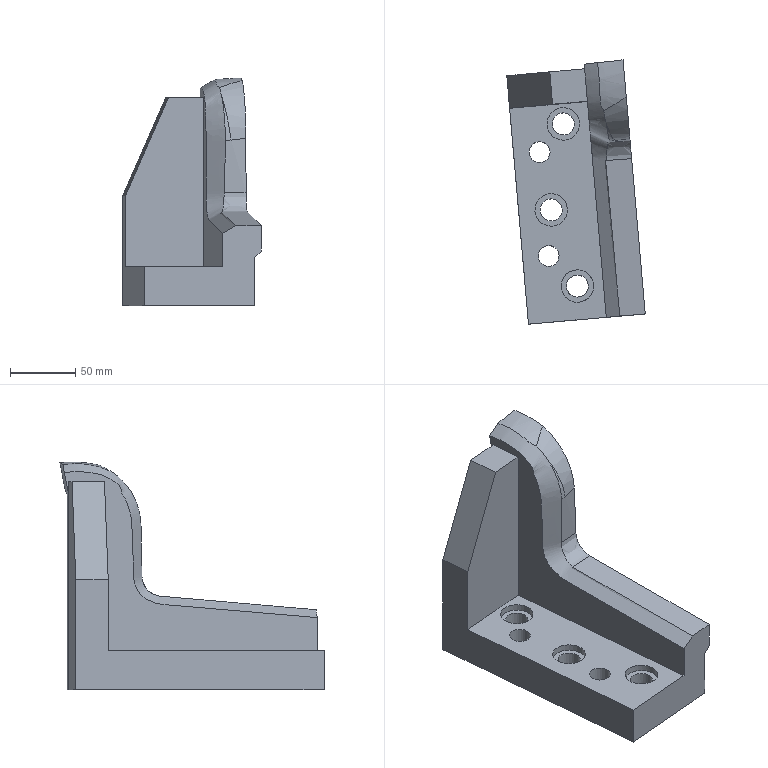Part | NX | features solid 2 | 1 solid | 33 faces | box 106.34 x 202.815 x 175.071 mm | volume 955587 mm3 | plane 14 | spline 11 | cylinder 8 | commonest cylinder face diameters 17 x3 25 x3 16 x2